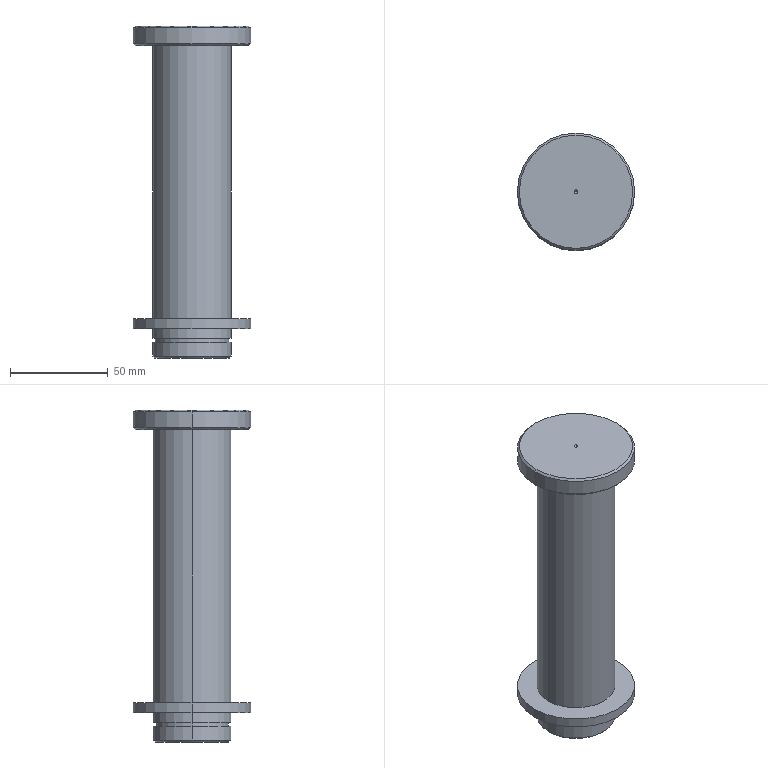Part | SolidWorks | features BaseBody 2 | 2 solids | 29 faces | box 60 x 60 x 170 mm | volume 236636 mm3 | cylinder 12 | cone 10 | plane 7 | commonest cylinder face diameters 40 x6 60 x4 37.5 x2
STEP:
#1=CARTESIAN_POINT('',(20.,0.,-89.));
#2=VERTEX_POINT('',#1);
#3=CARTESIAN_POINT('',(-20.,0.,-89.));
#4=VERTEX_POINT('',#3);
#5=CARTESIAN_POINT('',(0.,0.,-89.));
#6=DIRECTION('',(0.,0.,1.));
#7=DIRECTION('',(1.,0.,0.));
#8=AXIS2_PLACEMENT_3D('',#5,#6,#7);
#9=CIRCLE('',#8,20.);
#10=EDGE_CURVE('',#2,#4,#9,.T.);
#11=ORIENTED_EDGE('',*,*,#10,.T.);
#12=CARTESIAN_POINT('',(-20.,0.,-82.));
#13=VERTEX_POINT('',#12);
#14=CARTESIAN_POINT('',(-20.,0.,79.));
#15=DIRECTION('',(0.,0.,1.));
#16=VECTOR('',#15,1000.);
#17=LINE('',#14,#16);
#18=EDGE_CURVE('',#4,#13,#17,.T.);
#19=ORIENTED_EDGE('',*,*,#18,.T.);
#20=CARTESIAN_POINT('',(20.,0.,-82.));
#21=VERTEX_POINT('',#20);
#22=CARTESIAN_POINT('',(0.,0.,-82.));
#23=DIRECTION('',(0.,0.,1.));
#24=DIRECTION('',(1.,0.,0.));
#25=AXIS2_PLACEMENT_3D('',#22,#23,#24);
#26=CIRCLE('',#25,20.);
#27=EDGE_CURVE('',#21,#13,#26,.T.);
#28=ORIENTED_EDGE('',*,*,#27,.F.);
#29=CARTESIAN_POINT('',(20.,0.,79.));
#30=DIRECTION('',(0.,0.,1.));
#31=VECTOR('',#30,1000.);
#32=LINE('',#29,#31);
#33=EDGE_CURVE('',#2,#21,#32,.T.);
#34=ORIENTED_EDGE('',*,*,#33,.F.);
#35=EDGE_LOOP('',(#11,#19,#28,#34));
#36=FACE_OUTER_BOUND('',#35,.T.);
#37=CARTESIAN_POINT('',(0.,0.,79.));
#38=DIRECTION('',(0.,0.,1.));
#39=DIRECTION('',(1.,0.,0.));
#40=AXIS2_PLACEMENT_3D('',#37,#38,#39);
#41=CYLINDRICAL_SURFACE('',#40,20.);
#42=ADVANCED_FACE('',(#36),#41,.T.);
#43=CARTESIAN_POINT('',(19.,0.,-90.));
#44=VERTEX_POINT('',#43);
#45=CARTESIAN_POINT('',(-19.,0.,-90.));
#46=VERTEX_POINT('',#45);
#47=CARTESIAN_POINT('',(0.,0.,-90.));
#48=DIRECTION('',(0.,0.,1.));
#49=DIRECTION('',(1.,0.,0.));
#50=AXIS2_PLACEMENT_3D('',#47,#48,#49);
#51=CIRCLE('',#50,19.);
#52=EDGE_CURVE('',#44,#46,#51,.T.);
#53=ORIENTED_EDGE('',*,*,#52,.T.);
#54=CARTESIAN_POINT('',(-19.,0.,-90.));
#55=DIRECTION('',(-0.7071,0.,0.7071));
#56=VECTOR('',#55,1000.);
#57=LINE('',#54,#56);
#58=EDGE_CURVE('',#46,#4,#57,.T.);
#59=ORIENTED_EDGE('',*,*,#58,.T.);
#60=ORIENTED_EDGE('',*,*,#10,.F.);
#61=CARTESIAN_POINT('',(19.,0.,-90.));
#62=DIRECTION('',(0.7071,0.,0.7071));
#63=VECTOR('',#62,1000.);
#64=LINE('',#61,#63);
#65=EDGE_CURVE('',#44,#2,#64,.T.);
#66=ORIENTED_EDGE('',*,*,#65,.F.);
#67=EDGE_LOOP('',(#53,#59,#60,#66));
#68=FACE_OUTER_BOUND('',#67,.T.);
#69=CARTESIAN_POINT('',(0.,0.,-90.));
#70=DIRECTION('',(0.,0.,1.));
#71=DIRECTION('',(1.,0.,0.));
#72=AXIS2_PLACEMENT_3D('',#69,#70,#71);
#73=CONICAL_SURFACE('',#72,19.,0.7854);
#74=ADVANCED_FACE('',(#68),#73,.T.);
#75=CARTESIAN_POINT('',(0.,0.,-89.));
#76=VERTEX_POINT('',#75);
#77=CARTESIAN_POINT('',(-1.,0.,-90.));
#78=VERTEX_POINT('',#77);
#79=CARTESIAN_POINT('',(0.,0.,-89.));
#80=DIRECTION('',(-0.7071,0.,-0.7071));
#81=VECTOR('',#80,1000.);
#82=LINE('',#79,#81);
#83=EDGE_CURVE('',#76,#78,#82,.T.);
#84=ORIENTED_EDGE('',*,*,#83,.F.);
#85=CARTESIAN_POINT('',(1.,0.,-90.));
#86=VERTEX_POINT('',#85);
#87=CARTESIAN_POINT('',(0.,0.,-89.));
#88=DIRECTION('',(0.7071,0.,-0.7071));
#89=VECTOR('',#88,1000.);
#90=LINE('',#87,#89);
#91=EDGE_CURVE('',#76,#86,#90,.T.);
#92=ORIENTED_EDGE('',*,*,#91,.T.);
#93=CARTESIAN_POINT('',(0.,0.,-90.));
#94=DIRECTION('',(0.,0.,1.));
#95=DIRECTION('',(1.,0.,0.));
#96=AXIS2_PLACEMENT_3D('',#93,#94,#95);
#97=CIRCLE('',#96,1.);
#98=EDGE_CURVE('',#78,#86,#97,.T.);
#99=ORIENTED_EDGE('',*,*,#98,.F.);
#100=EDGE_LOOP('',(#84,#92,#99));
#101=FACE_OUTER_BOUND('',#100,.T.);
#102=CARTESIAN_POINT('',(0.,0.,-1089.));
#103=DIRECTION('',(0.,0.,-1.));
#104=DIRECTION('',(-1.,0.,0.));
#105=AXIS2_PLACEMENT_3D('',#102,#103,#104);
#106=CONICAL_SURFACE('',#105,1000.,0.7854);
#107=ADVANCED_FACE('',(#101),#106,.F.);
#108=CARTESIAN_POINT('',(0.,0.,79.));
#109=VERTEX_POINT('',#108);
#110=CARTESIAN_POINT('',(1.,0.,80.));
#111=VERTEX_POINT('',#110);
#112=CARTESIAN_POINT('',(1.,0.,80.));
#113=DIRECTION('',(0.7071,0.,0.7071));
#114=VECTOR('',#113,1000.);
#115=LINE('',#112,#114);
#116=EDGE_CURVE('',#109,#111,#115,.T.);
#117=ORIENTED_EDGE('',*,*,#116,.F.);
#118=CARTESIAN_POINT('',(-1.,0.,80.));
#119=VERTEX_POINT('',#118);
#120=CARTESIAN_POINT('',(-1.,0.,80.));
#121=DIRECTION('',(-0.7071,0.,0.7071));
#122=VECTOR('',#121,1000.);
#123=LINE('',#120,#122);
#124=EDGE_CURVE('',#109,#119,#123,.T.);
#125=ORIENTED_EDGE('',*,*,#124,.T.);
#126=CARTESIAN_POINT('',(0.,0.,80.));
#127=DIRECTION('',(0.,0.,1.));
#128=DIRECTION('',(1.,0.,0.));
#129=AXIS2_PLACEMENT_3D('',#126,#127,#128);
#130=CIRCLE('',#129,1.);
#131=EDGE_CURVE('',#119,#111,#130,.T.);
#132=ORIENTED_EDGE('',*,*,#131,.T.);
#133=EDGE_LOOP('',(#117,#125,#132));
#134=FACE_OUTER_BOUND('',#133,.T.);
#135=CARTESIAN_POINT('',(0.,0.,80.));
#136=DIRECTION('',(0.,0.,1.));
#137=DIRECTION('',(1.,0.,0.));
#138=AXIS2_PLACEMENT_3D('',#135,#136,#137);
#139=CONICAL_SURFACE('',#138,1.,0.7854);
#140=ADVANCED_FACE('',(#134),#139,.F.);
#141=CARTESIAN_POINT('',(29.,0.,80.));
#142=VERTEX_POINT('',#141);
#143=CARTESIAN_POINT('',(-29.,0.,80.));
#144=VERTEX_POINT('',#143);
#145=CARTESIAN_POINT('',(0.,0.,80.));
#146=DIRECTION('',(0.,0.,1.));
#147=DIRECTION('',(1.,0.,0.));
#148=AXIS2_PLACEMENT_3D('',#145,#146,#147);
#149=CIRCLE('',#148,29.);
#150=EDGE_CURVE('',#142,#144,#149,.T.);
#151=ORIENTED_EDGE('',*,*,#150,.F.);
#152=CARTESIAN_POINT('',(30.,0.,79.));
#153=VERTEX_POINT('',#152);
#154=CARTESIAN_POINT('',(30.,0.,79.));
#155=DIRECTION('',(0.7071,0.,-0.7071));
#156=VECTOR('',#155,1000.);
#157=LINE('',#154,#156);
#158=EDGE_CURVE('',#142,#153,#157,.T.);
#159=ORIENTED_EDGE('',*,*,#158,.T.);
#160=CARTESIAN_POINT('',(-30.,0.,79.));
#161=VERTEX_POINT('',#160);
#162=CARTESIAN_POINT('',(0.,0.,79.));
#163=DIRECTION('',(0.,0.,1.));
#164=DIRECTION('',(1.,0.,0.));
#165=AXIS2_PLACEMENT_3D('',#162,#163,#164);
#166=CIRCLE('',#165,30.);
#167=EDGE_CURVE('',#153,#161,#166,.T.);
#168=ORIENTED_EDGE('',*,*,#167,.T.);
#169=CARTESIAN_POINT('',(-30.,0.,79.));
#170=DIRECTION('',(-0.7071,0.,-0.7071));
#171=VECTOR('',#170,1000.);
#172=LINE('',#169,#171);
#173=EDGE_CURVE('',#144,#161,#172,.T.);
#174=ORIENTED_EDGE('',*,*,#173,.F.);
#175=EDGE_LOOP('',(#151,#159,#168,#174));
#176=FACE_OUTER_BOUND('',#175,.T.);
#177=CARTESIAN_POINT('',(0.,0.,79.));
#178=DIRECTION('',(0.,0.,-1.));
#179=DIRECTION('',(-1.,0.,0.));
#180=AXIS2_PLACEMENT_3D('',#177,#178,#179);
#181=CONICAL_SURFACE('',#180,30.,0.7854);
#182=ADVANCED_FACE('',(#176),#181,.T.);
#183=CARTESIAN_POINT('',(30.,0.,71.));
#184=VERTEX_POINT('',#183);
#185=CARTESIAN_POINT('',(-30.,0.,71.));
#186=VERTEX_POINT('',#185);
#187=CARTESIAN_POINT('',(0.,0.,71.));
#188=DIRECTION('',(0.,0.,1.));
#189=DIRECTION('',(1.,0.,0.));
#190=AXIS2_PLACEMENT_3D('',#187,#188,#189);
#191=CIRCLE('',#190,30.);
#192=EDGE_CURVE('',#184,#186,#191,.T.);
#193=ORIENTED_EDGE('',*,*,#192,.T.);
#194=CARTESIAN_POINT('',(-30.,0.,79.));
#195=DIRECTION('',(0.,0.,1.));
#196=VECTOR('',#195,1000.);
#197=LINE('',#194,#196);
#198=EDGE_CURVE('',#186,#161,#197,.T.);
#199=ORIENTED_EDGE('',*,*,#198,.T.);
#200=ORIENTED_EDGE('',*,*,#167,.F.);
#201=CARTESIAN_POINT('',(30.,0.,79.));
#202=DIRECTION('',(0.,0.,1.));
#203=VECTOR('',#202,1000.);
#204=LINE('',#201,#203);
#205=EDGE_CURVE('',#184,#153,#204,.T.);
#206=ORIENTED_EDGE('',*,*,#205,.F.);
#207=EDGE_LOOP('',(#193,#199,#200,#206));
#208=FACE_OUTER_BOUND('',#207,.T.);
#209=CARTESIAN_POINT('',(0.,0.,79.));
#210=DIRECTION('',(0.,0.,1.));
#211=DIRECTION('',(1.,0.,0.));
#212=AXIS2_PLACEMENT_3D('',#209,#210,#211);
#213=CYLINDRICAL_SURFACE('',#212,30.);
#214=ADVANCED_FACE('',(#208),#213,.T.);
#215=CARTESIAN_POINT('',(29.,0.,70.));
#216=VERTEX_POINT('',#215);
#217=CARTESIAN_POINT('',(-29.,0.,70.));
#218=VERTEX_POINT('',#217);
#219=CARTESIAN_POINT('',(0.,0.,70.));
#220=DIRECTION('',(0.,0.,1.));
#221=DIRECTION('',(1.,0.,0.));
#222=AXIS2_PLACEMENT_3D('',#219,#220,#221);
#223=CIRCLE('',#222,29.);
#224=EDGE_CURVE('',#216,#218,#223,.T.);
#225=ORIENTED_EDGE('',*,*,#224,.T.);
#226=CARTESIAN_POINT('',(-29.,0.,70.));
#227=DIRECTION('',(-0.7071,0.,0.7071));
#228=VECTOR('',#227,1000.);
#229=LINE('',#226,#228);
#230=EDGE_CURVE('',#218,#186,#229,.T.);
#231=ORIENTED_EDGE('',*,*,#230,.T.);
#232=ORIENTED_EDGE('',*,*,#192,.F.);
#233=CARTESIAN_POINT('',(29.,0.,70.));
#234=DIRECTION('',(0.7071,0.,0.7071));
#235=VECTOR('',#234,1000.);
#236=LINE('',#233,#235);
#237=EDGE_CURVE('',#216,#184,#236,.T.);
#238=ORIENTED_EDGE('',*,*,#237,.F.);
#239=EDGE_LOOP('',(#225,#231,#232,#238));
#240=FACE_OUTER_BOUND('',#239,.T.);
#241=CARTESIAN_POINT('',(0.,0.,70.));
#242=DIRECTION('',(0.,0.,1.));
#243=DIRECTION('',(1.,0.,0.));
#244=AXIS2_PLACEMENT_3D('',#241,#242,#243);
#245=CONICAL_SURFACE('',#244,29.,0.7854);
#246=ADVANCED_FACE('',(#240),#245,.T.);
#247=CARTESIAN_POINT('',(20.,0.,-80.));
#248=VERTEX_POINT('',#247);
#249=CARTESIAN_POINT('',(-20.,0.,-80.));
#250=VERTEX_POINT('',#249);
#251=CARTESIAN_POINT('',(0.,0.,-80.));
#252=DIRECTION('',(0.,0.,1.));
#253=DIRECTION('',(1.,0.,0.));
#254=AXIS2_PLACEMENT_3D('',#251,#252,#253);
#255=CIRCLE('',#254,20.);
#256=EDGE_CURVE('',#248,#250,#255,.T.);
#257=ORIENTED_EDGE('',*,*,#256,.T.);
#258=CARTESIAN_POINT('',(-20.,0.,70.));
#259=VERTEX_POINT('',#258);
#260=CARTESIAN_POINT('',(-20.,0.,79.));
#261=DIRECTION('',(0.,0.,1.));
#262=VECTOR('',#261,1000.);
#263=LINE('',#260,#262);
#264=EDGE_CURVE('',#250,#259,#263,.T.);
#265=ORIENTED_EDGE('',*,*,#264,.T.);
#266=CARTESIAN_POINT('',(20.,0.,70.));
#267=VERTEX_POINT('',#266);
#268=CARTESIAN_POINT('',(0.,0.,70.));
#269=DIRECTION('',(0.,0.,1.));
#270=DIRECTION('',(1.,0.,0.));
#271=AXIS2_PLACEMENT_3D('',#268,#269,#270);
#272=CIRCLE('',#271,20.);
#273=EDGE_CURVE('',#267,#259,#272,.T.);
#274=ORIENTED_EDGE('',*,*,#273,.F.);
#275=CARTESIAN_POINT('',(20.,0.,79.));
#276=DIRECTION('',(0.,0.,1.));
#277=VECTOR('',#276,1000.);
#278=LINE('',#275,#277);
#279=EDGE_CURVE('',#248,#267,#278,.T.);
#280=ORIENTED_EDGE('',*,*,#279,.F.);
#281=EDGE_LOOP('',(#257,#265,#274,#280));
#282=FACE_OUTER_BOUND('',#281,.T.);
#283=CARTESIAN_POINT('',(0.,0.,79.));
#284=DIRECTION('',(0.,0.,1.));
#285=DIRECTION('',(1.,0.,0.));
#286=AXIS2_PLACEMENT_3D('',#283,#284,#285);
#287=CYLINDRICAL_SURFACE('',#286,20.);
#288=ADVANCED_FACE('',(#282),#287,.T.);
#289=CARTESIAN_POINT('',(18.75,0.,-82.));
#290=VERTEX_POINT('',#289);
#291=CARTESIAN_POINT('',(-18.75,0.,-82.));
#292=VERTEX_POINT('',#291);
#293=CARTESIAN_POINT('',(0.,0.,-82.));
#294=DIRECTION('',(0.,0.,1.));
#295=DIRECTION('',(1.,0.,0.));
#296=AXIS2_PLACEMENT_3D('',#293,#294,#295);
#297=CIRCLE('',#296,18.75);
#298=EDGE_CURVE('',#290,#292,#297,.T.);
#299=ORIENTED_EDGE('',*,*,#298,.T.);
#300=CARTESIAN_POINT('',(-18.75,0.,-80.));
#301=VERTEX_POINT('',#300);
#302=CARTESIAN_POINT('',(-18.75,0.,79.));
#303=DIRECTION('',(0.,0.,1.));
#304=VECTOR('',#303,1000.);
#305=LINE('',#302,#304);
#306=EDGE_CURVE('',#292,#301,#305,.T.);
#307=ORIENTED_EDGE('',*,*,#306,.T.);
#308=CARTESIAN_POINT('',(18.75,0.,-80.));
#309=VERTEX_POINT('',#308);
#310=CARTESIAN_POINT('',(0.,0.,-80.));
#311=DIRECTION('',(0.,0.,1.));
#312=DIRECTION('',(1.,0.,0.));
#313=AXIS2_PLACEMENT_3D('',#310,#311,#312);
#314=CIRCLE('',#313,18.75);
#315=EDGE_CURVE('',#309,#301,#314,.T.);
#316=ORIENTED_EDGE('',*,*,#315,.F.);
#317=CARTESIAN_POINT('',(18.75,0.,79.));
#318=DIRECTION('',(0.,0.,1.));
#319=VECTOR('',#318,1000.);
#320=LINE('',#317,#319);
#321=EDGE_CURVE('',#290,#309,#320,.T.);
#322=ORIENTED_EDGE('',*,*,#321,.F.);
#323=EDGE_LOOP('',(#299,#307,#316,#322));
#324=FACE_OUTER_BOUND('',#323,.T.);
#325=CARTESIAN_POINT('',(0.,0.,79.));
#326=DIRECTION('',(0.,0.,1.));
#327=DIRECTION('',(1.,0.,0.));
#328=AXIS2_PLACEMENT_3D('',#325,#326,#327);
#329=CYLINDRICAL_SURFACE('',#328,18.75);
#330=ADVANCED_FACE('',(#324),#329,.T.);
#331=ORIENTED_EDGE('',*,*,#306,.F.);
#332=CARTESIAN_POINT('',(0.,0.,-82.));
#333=DIRECTION('',(0.,0.,1.));
#334=DIRECTION('',(1.,0.,0.));
#335=AXIS2_PLACEMENT_3D('',#332,#333,#334);
#336=CIRCLE('',#335,18.75);
#337=EDGE_CURVE('',#292,#290,#336,.T.);
#338=ORIENTED_EDGE('',*,*,#337,.T.);
#339=ORIENTED_EDGE('',*,*,#321,.T.);
#340=CARTESIAN_POINT('',(0.,0.,-80.));
#341=DIRECTION('',(0.,0.,1.));
#342=DIRECTION('',(1.,0.,0.));
#343=AXIS2_PLACEMENT_3D('',#340,#341,#342);
#344=CIRCLE('',#343,18.75);
#345=EDGE_CURVE('',#301,#309,#344,.T.);
#346=ORIENTED_EDGE('',*,*,#345,.F.);
#347=EDGE_LOOP('',(#331,#338,#339,#346));
#348=FACE_OUTER_BOUND('',#347,.T.);
#349=CARTESIAN_POINT('',(0.,0.,79.));
#350=DIRECTION('',(0.,0.,1.));
#351=DIRECTION('',(1.,0.,0.));
#352=AXIS2_PLACEMENT_3D('',#349,#350,#351);
#353=CYLINDRICAL_SURFACE('',#352,18.75);
#354=ADVANCED_FACE('',(#348),#353,.T.);
#355=ORIENTED_EDGE('',*,*,#256,.F.);
#356=CARTESIAN_POINT('',(0.,0.,-80.));
#357=DIRECTION('',(0.,0.,1.));
#358=DIRECTION('',(1.,0.,0.));
#359=AXIS2_PLACEMENT_3D('',#356,#357,#358);
#360=CIRCLE('',#359,20.);
#361=EDGE_CURVE('',#250,#248,#360,.T.);
#362=ORIENTED_EDGE('',*,*,#361,.F.);
#363=EDGE_LOOP('',(#355,#362));
#364=FACE_OUTER_BOUND('',#363,.T.);
#365=ORIENTED_EDGE('',*,*,#315,.T.);
#366=ORIENTED_EDGE('',*,*,#345,.T.);
#367=EDGE_LOOP('',(#365,#366));
#368=FACE_BOUND('',#367,.T.);
#369=CARTESIAN_POINT('',(0.,20.,-80.));
#370=DIRECTION('',(0.,0.,1.));
#371=DIRECTION('',(1.,0.,0.));
#372=AXIS2_PLACEMENT_3D('',#369,#370,#371);
#373=PLANE('',#372);
#374=ADVANCED_FACE('',(#364,#368),#373,.F.);
#375=ORIENTED_EDGE('',*,*,#264,.F.);
#376=ORIENTED_EDGE('',*,*,#361,.T.);
#377=ORIENTED_EDGE('',*,*,#279,.T.);
#378=CARTESIAN_POINT('',(0.,0.,70.));
#379=DIRECTION('',(0.,0.,1.));
#380=DIRECTION('',(1.,0.,0.));
#381=AXIS2_PLACEMENT_3D('',#378,#379,#380);
#382=CIRCLE('',#381,20.);
#383=EDGE_CURVE('',#259,#267,#382,.T.);
#384=ORIENTED_EDGE('',*,*,#383,.F.);
#385=EDGE_LOOP('',(#375,#376,#377,#384));
#386=FACE_OUTER_BOUND('',#385,.T.);
#387=CARTESIAN_POINT('',(0.,0.,79.));
#388=DIRECTION('',(0.,0.,1.));
#389=DIRECTION('',(1.,0.,0.));
#390=AXIS2_PLACEMENT_3D('',#387,#388,#389);
#391=CYLINDRICAL_SURFACE('',#390,20.);
#392=ADVANCED_FACE('',(#386),#391,.T.);
#393=ORIENTED_EDGE('',*,*,#224,.F.);
#394=CARTESIAN_POINT('',(0.,0.,70.));
#395=DIRECTION('',(0.,0.,1.));
#396=DIRECTION('',(1.,0.,0.));
#397=AXIS2_PLACEMENT_3D('',#394,#395,#396);
#398=CIRCLE('',#397,29.);
#399=EDGE_CURVE('',#218,#216,#398,.T.);
#400=ORIENTED_EDGE('',*,*,#399,.F.);
#401=EDGE_LOOP('',(#393,#400));
#402=FACE_OUTER_BOUND('',#401,.T.);
#403=ORIENTED_EDGE('',*,*,#273,.T.);
#404=ORIENTED_EDGE('',*,*,#383,.T.);
#405=EDGE_LOOP('',(#403,#404));
#406=FACE_BOUND('',#405,.T.);
#407=CARTESIAN_POINT('',(0.,29.,70.));
#408=DIRECTION('',(0.,0.,1.));
#409=DIRECTION('',(1.,0.,0.));
#410=AXIS2_PLACEMENT_3D('',#407,#408,#409);
#411=PLANE('',#410);
#412=ADVANCED_FACE('',(#402,#406),#411,.F.);
#413=ORIENTED_EDGE('',*,*,#230,.F.);
#414=ORIENTED_EDGE('',*,*,#399,.T.);
#415=ORIENTED_EDGE('',*,*,#237,.T.);
#416=CARTESIAN_POINT('',(0.,0.,71.));
#417=DIRECTION('',(0.,0.,1.));
#418=DIRECTION('',(1.,0.,0.));
#419=AXIS2_PLACEMENT_3D('',#416,#417,#418);
#420=CIRCLE('',#419,30.);
#421=EDGE_CURVE('',#186,#184,#420,.T.);
#422=ORIENTED_EDGE('',*,*,#421,.F.);
#423=EDGE_LOOP('',(#413,#414,#415,#422));
#424=FACE_OUTER_BOUND('',#423,.T.);
#425=CARTESIAN_POINT('',(0.,0.,70.));
#426=DIRECTION('',(0.,0.,1.));
#427=DIRECTION('',(1.,0.,0.));
#428=AXIS2_PLACEMENT_3D('',#425,#426,#427);
#429=CONICAL_SURFACE('',#428,29.,0.7854);
#430=ADVANCED_FACE('',(#424),#429,.T.);
#431=ORIENTED_EDGE('',*,*,#198,.F.);
#432=ORIENTED_EDGE('',*,*,#421,.T.);
#433=ORIENTED_EDGE('',*,*,#205,.T.);
#434=CARTESIAN_POINT('',(0.,0.,79.));
#435=DIRECTION('',(0.,0.,1.));
#436=DIRECTION('',(1.,0.,0.));
#437=AXIS2_PLACEMENT_3D('',#434,#435,#436);
#438=CIRCLE('',#437,30.);
#439=EDGE_CURVE('',#161,#153,#438,.T.);
#440=ORIENTED_EDGE('',*,*,#439,.F.);
#441=EDGE_LOOP('',(#431,#432,#433,#440));
#442=FACE_OUTER_BOUND('',#441,.T.);
#443=CARTESIAN_POINT('',(0.,0.,79.));
#444=DIRECTION('',(0.,0.,1.));
#445=DIRECTION('',(1.,0.,0.));
#446=AXIS2_PLACEMENT_3D('',#443,#444,#445);
#447=CYLINDRICAL_SURFACE('',#446,30.);
#448=ADVANCED_FACE('',(#442),#447,.T.);
#449=ORIENTED_EDGE('',*,*,#158,.F.);
#450=CARTESIAN_POINT('',(0.,0.,80.));
#451=DIRECTION('',(0.,0.,1.));
#452=DIRECTION('',(1.,0.,0.));
#453=AXIS2_PLACEMENT_3D('',#450,#451,#452);
#454=CIRCLE('',#453,29.);
#455=EDGE_CURVE('',#144,#142,#454,.T.);
#456=ORIENTED_EDGE('',*,*,#455,.F.);
#457=ORIENTED_EDGE('',*,*,#173,.T.);
#458=ORIENTED_EDGE('',*,*,#439,.T.);
#459=EDGE_LOOP('',(#449,#456,#457,#458));
#460=FACE_OUTER_BOUND('',#459,.T.);
#461=CARTESIAN_POINT('',(0.,0.,79.));
#462=DIRECTION('',(0.,0.,-1.));
#463=DIRECTION('',(-1.,0.,0.));
#464=AXIS2_PLACEMENT_3D('',#461,#462,#463);
#465=CONICAL_SURFACE('',#464,30.,0.7854);
#466=ADVANCED_FACE('',(#460),#465,.T.);
#467=CARTESIAN_POINT('',(0.,0.,80.));
#468=DIRECTION('',(0.,0.,1.));
#469=DIRECTION('',(1.,0.,0.));
#470=AXIS2_PLACEMENT_3D('',#467,#468,#469);
#471=CIRCLE('',#470,1.);
#472=EDGE_CURVE('',#111,#119,#471,.T.);
#473=ORIENTED_EDGE('',*,*,#472,.F.);
#474=ORIENTED_EDGE('',*,*,#131,.F.);
#475=EDGE_LOOP('',(#473,#474));
#476=FACE_BOUND('',#475,.T.);
#477=ORIENTED_EDGE('',*,*,#455,.T.);
#478=ORIENTED_EDGE('',*,*,#150,.T.);
#479=EDGE_LOOP('',(#477,#478));
#480=FACE_OUTER_BOUND('',#479,.T.);
#481=CARTESIAN_POINT('',(0.,1.,80.));
#482=DIRECTION('',(0.,0.,-1.));
#483=DIRECTION('',(-1.,0.,0.));
#484=AXIS2_PLACEMENT_3D('',#481,#482,#483);
#485=PLANE('',#484);
#486=ADVANCED_FACE('',(#476,#480),#485,.F.);
#487=ORIENTED_EDGE('',*,*,#124,.F.);
#488=ORIENTED_EDGE('',*,*,#116,.T.);
#489=ORIENTED_EDGE('',*,*,#472,.T.);
#490=EDGE_LOOP('',(#487,#488,#489));
#491=FACE_OUTER_BOUND('',#490,.T.);
#492=CARTESIAN_POINT('',(0.,0.,80.));
#493=DIRECTION('',(0.,0.,1.));
#494=DIRECTION('',(1.,0.,0.));
#495=AXIS2_PLACEMENT_3D('',#492,#493,#494);
#496=CONICAL_SURFACE('',#495,1.,0.7854);
#497=ADVANCED_FACE('',(#491),#496,.F.);
#498=ORIENTED_EDGE('',*,*,#91,.F.);
#499=ORIENTED_EDGE('',*,*,#83,.T.);
#500=CARTESIAN_POINT('',(0.,0.,-90.));
#501=DIRECTION('',(0.,0.,1.));
#502=DIRECTION('',(1.,0.,0.));
#503=AXIS2_PLACEMENT_3D('',#500,#501,#502);
#504=CIRCLE('',#503,1.);
#505=EDGE_CURVE('',#86,#78,#504,.T.);
#506=ORIENTED_EDGE('',*,*,#505,.F.);
#507=EDGE_LOOP('',(#498,#499,#506));
#508=FACE_OUTER_BOUND('',#507,.T.);
#509=CARTESIAN_POINT('',(0.,0.,-1089.));
#510=DIRECTION('',(0.,0.,-1.));
#511=DIRECTION('',(-1.,0.,0.));
#512=AXIS2_PLACEMENT_3D('',#509,#510,#511);
#513=CONICAL_SURFACE('',#512,1000.,0.7854);
#514=ADVANCED_FACE('',(#508),#513,.F.);
#515=ORIENTED_EDGE('',*,*,#52,.F.);
#516=CARTESIAN_POINT('',(0.,0.,-90.));
#517=DIRECTION('',(0.,0.,1.));
#518=DIRECTION('',(1.,0.,0.));
#519=AXIS2_PLACEMENT_3D('',#516,#517,#518);
#520=CIRCLE('',#519,19.);
#521=EDGE_CURVE('',#46,#44,#520,.T.);
#522=ORIENTED_EDGE('',*,*,#521,.F.);
#523=EDGE_LOOP('',(#515,#522));
#524=FACE_OUTER_BOUND('',#523,.T.);
#525=ORIENTED_EDGE('',*,*,#98,.T.);
#526=ORIENTED_EDGE('',*,*,#505,.T.);
#527=EDGE_LOOP('',(#525,#526));
#528=FACE_BOUND('',#527,.T.);
#529=CARTESIAN_POINT('',(0.,19.,-90.));
#530=DIRECTION('',(0.,0.,1.));
#531=DIRECTION('',(1.,0.,0.));
#532=AXIS2_PLACEMENT_3D('',#529,#530,#531);
#533=PLANE('',#532);
#534=ADVANCED_FACE('',(#524,#528),#533,.F.);
#535=ORIENTED_EDGE('',*,*,#58,.F.);
#536=ORIENTED_EDGE('',*,*,#521,.T.);
#537=ORIENTED_EDGE('',*,*,#65,.T.);
#538=CARTESIAN_POINT('',(0.,0.,-89.));
#539=DIRECTION('',(0.,0.,1.));
#540=DIRECTION('',(1.,0.,0.));
#541=AXIS2_PLACEMENT_3D('',#538,#539,#540);
#542=CIRCLE('',#541,20.);
#543=EDGE_CURVE('',#4,#2,#542,.T.);
#544=ORIENTED_EDGE('',*,*,#543,.F.);
#545=EDGE_LOOP('',(#535,#536,#537,#544));
#546=FACE_OUTER_BOUND('',#545,.T.);
#547=CARTESIAN_POINT('',(0.,0.,-90.));
#548=DIRECTION('',(0.,0.,1.));
#549=DIRECTION('',(1.,0.,0.));
#550=AXIS2_PLACEMENT_3D('',#547,#548,#549);
#551=CONICAL_SURFACE('',#550,19.,0.7854);
#552=ADVANCED_FACE('',(#546),#551,.T.);
#553=ORIENTED_EDGE('',*,*,#18,.F.);
#554=ORIENTED_EDGE('',*,*,#543,.T.);
#555=ORIENTED_EDGE('',*,*,#33,.T.);
#556=CARTESIAN_POINT('',(0.,0.,-82.));
#557=DIRECTION('',(0.,0.,1.));
#558=DIRECTION('',(1.,0.,0.));
#559=AXIS2_PLACEMENT_3D('',#556,#557,#558);
#560=CIRCLE('',#559,20.);
#561=EDGE_CURVE('',#13,#21,#560,.T.);
#562=ORIENTED_EDGE('',*,*,#561,.F.);
#563=EDGE_LOOP('',(#553,#554,#555,#562));
#564=FACE_OUTER_BOUND('',#563,.T.);
#565=CARTESIAN_POINT('',(0.,0.,79.));
#566=DIRECTION('',(0.,0.,1.));
#567=DIRECTION('',(1.,0.,0.));
#568=AXIS2_PLACEMENT_3D('',#565,#566,#567);
#569=CYLINDRICAL_SURFACE('',#568,20.);
#570=ADVANCED_FACE('',(#564),#569,.T.);
#571=ORIENTED_EDGE('',*,*,#298,.F.);
#572=ORIENTED_EDGE('',*,*,#337,.F.);
#573=EDGE_LOOP('',(#571,#572));
#574=FACE_BOUND('',#573,.T.);
#575=ORIENTED_EDGE('',*,*,#27,.T.);
#576=ORIENTED_EDGE('',*,*,#561,.T.);
#577=EDGE_LOOP('',(#575,#576));
#578=FACE_OUTER_BOUND('',#577,.T.);
#579=CARTESIAN_POINT('',(0.,18.75,-82.));
#580=DIRECTION('',(0.,0.,-1.));
#581=DIRECTION('',(-1.,0.,0.));
#582=AXIS2_PLACEMENT_3D('',#579,#580,#581);
#583=PLANE('',#582);
#584=ADVANCED_FACE('',(#574,#578),#583,.F.);
#585=CLOSED_SHELL('',(#42,#74,#107,#140,#182,#214,#246,#288,#330,#354,#374,#392,#412,#430,#448,#466,#486,#497,#514,#534,#552,#570,#584));
#586=MANIFOLD_SOLID_BREP('',#585);
#587=CARTESIAN_POINT('',(20.,0.,-70.));
#588=VERTEX_POINT('',#587);
#589=CARTESIAN_POINT('',(-20.,0.,-70.));
#590=VERTEX_POINT('',#589);
#591=CARTESIAN_POINT('',(0.,0.,-70.));
#592=DIRECTION('',(0.,0.,-1.));
#593=DIRECTION('',(-1.,0.,0.));
#594=AXIS2_PLACEMENT_3D('',#591,#592,#593);
#595=CIRCLE('',#594,20.);
#596=EDGE_CURVE('',#588,#590,#595,.T.);
#597=ORIENTED_EDGE('',*,*,#596,.F.);
#598=CARTESIAN_POINT('',(20.,0.,-75.));
#599=VERTEX_POINT('',#598);
#600=CARTESIAN_POINT('',(20.,0.,-70.));
#601=DIRECTION('',(0.,0.,-1.));
#602=VECTOR('',#601,1000.);
#603=LINE('',#600,#602);
#604=EDGE_CURVE('',#588,#599,#603,.T.);
#605=ORIENTED_EDGE('',*,*,#604,.T.);
#606=CARTESIAN_POINT('',(-20.,0.,-75.));
#607=VERTEX_POINT('',#606);
#608=CARTESIAN_POINT('',(0.,0.,-75.));
#609=DIRECTION('',(0.,0.,-1.));
#610=DIRECTION('',(-1.,0.,0.));
#611=AXIS2_PLACEMENT_3D('',#608,#609,#610);
#612=CIRCLE('',#611,20.);
#613=EDGE_CURVE('',#599,#607,#612,.T.);
#614=ORIENTED_EDGE('',*,*,#613,.T.);
#615=CARTESIAN_POINT('',(-20.,0.,-70.));
#616=DIRECTION('',(0.,0.,-1.));
#617=VECTOR('',#616,1000.);
#618=LINE('',#615,#617);
#619=EDGE_CURVE('',#590,#607,#618,.T.);
#620=ORIENTED_EDGE('',*,*,#619,.F.);
#621=EDGE_LOOP('',(#597,#605,#614,#620));
#622=FACE_OUTER_BOUND('',#621,.T.);
#623=CARTESIAN_POINT('',(0.,0.,-70.));
#624=DIRECTION('',(0.,0.,-1.));
#625=DIRECTION('',(-1.,0.,0.));
#626=AXIS2_PLACEMENT_3D('',#623,#624,#625);
#627=CYLINDRICAL_SURFACE('',#626,20.);
#628=ADVANCED_FACE('',(#622),#627,.F.);
#629=CARTESIAN_POINT('',(-30.,0.,-70.));
#630=VERTEX_POINT('',#629);
#631=CARTESIAN_POINT('',(30.,0.,-70.));
#632=VERTEX_POINT('',#631);
#633=CARTESIAN_POINT('',(0.,0.,-70.));
#634=DIRECTION('',(0.,0.,-1.));
#635=DIRECTION('',(-1.,0.,0.));
#636=AXIS2_PLACEMENT_3D('',#633,#634,#635);
#637=CIRCLE('',#636,30.);
#638=EDGE_CURVE('',#630,#632,#637,.T.);
#639=ORIENTED_EDGE('',*,*,#638,.T.);
#640=CARTESIAN_POINT('',(30.,0.,-75.));
#641=VERTEX_POINT('',#640);
#642=CARTESIAN_POINT('',(30.,0.,-70.));
#643=DIRECTION('',(0.,0.,-1.));
#644=VECTOR('',#643,1000.);
#645=LINE('',#642,#644);
#646=EDGE_CURVE('',#632,#641,#645,.T.);
#647=ORIENTED_EDGE('',*,*,#646,.T.);
#648=CARTESIAN_POINT('',(-30.,0.,-75.));
#649=VERTEX_POINT('',#648);
#650=CARTESIAN_POINT('',(0.,0.,-75.));
#651=DIRECTION('',(0.,0.,-1.));
#652=DIRECTION('',(-1.,0.,0.));
#653=AXIS2_PLACEMENT_3D('',#650,#651,#652);
#654=CIRCLE('',#653,30.);
#655=EDGE_CURVE('',#649,#641,#654,.T.);
#656=ORIENTED_EDGE('',*,*,#655,.F.);
#657=CARTESIAN_POINT('',(-30.,0.,-70.));
#658=DIRECTION('',(0.,0.,-1.));
#659=VECTOR('',#658,1000.);
#660=LINE('',#657,#659);
#661=EDGE_CURVE('',#630,#649,#660,.T.);
#662=ORIENTED_EDGE('',*,*,#661,.F.);
#663=EDGE_LOOP('',(#639,#647,#656,#662));
#664=FACE_OUTER_BOUND('',#663,.T.);
#665=CARTESIAN_POINT('',(0.,0.,-70.));
#666=DIRECTION('',(0.,0.,-1.));
#667=DIRECTION('',(-1.,0.,0.));
#668=AXIS2_PLACEMENT_3D('',#665,#666,#667);
#669=CYLINDRICAL_SURFACE('',#668,30.);
#670=ADVANCED_FACE('',(#664),#669,.T.);
#671=ORIENTED_EDGE('',*,*,#646,.F.);
#672=CARTESIAN_POINT('',(0.,0.,-70.));
#673=DIRECTION('',(0.,0.,-1.));
#674=DIRECTION('',(-1.,0.,0.));
#675=AXIS2_PLACEMENT_3D('',#672,#673,#674);
#676=CIRCLE('',#675,30.);
#677=EDGE_CURVE('',#632,#630,#676,.T.);
#678=ORIENTED_EDGE('',*,*,#677,.T.);
#679=ORIENTED_EDGE('',*,*,#661,.T.);
#680=CARTESIAN_POINT('',(0.,0.,-75.));
#681=DIRECTION('',(0.,0.,-1.));
#682=DIRECTION('',(-1.,0.,0.));
#683=AXIS2_PLACEMENT_3D('',#680,#681,#682);
#684=CIRCLE('',#683,30.);
#685=EDGE_CURVE('',#641,#649,#684,.T.);
#686=ORIENTED_EDGE('',*,*,#685,.F.);
#687=EDGE_LOOP('',(#671,#678,#679,#686));
#688=FACE_OUTER_BOUND('',#687,.T.);
#689=CARTESIAN_POINT('',(0.,0.,-70.));
#690=DIRECTION('',(0.,0.,-1.));
#691=DIRECTION('',(-1.,0.,0.));
#692=AXIS2_PLACEMENT_3D('',#689,#690,#691);
#693=CYLINDRICAL_SURFACE('',#692,30.);
#694=ADVANCED_FACE('',(#688),#693,.T.);
#695=CARTESIAN_POINT('',(0.,0.,-70.));
#696=DIRECTION('',(0.,0.,-1.));
#697=DIRECTION('',(-1.,0.,0.));
#698=AXIS2_PLACEMENT_3D('',#695,#696,#697);
#699=CIRCLE('',#698,20.);
#700=EDGE_CURVE('',#590,#588,#699,.T.);
#701=ORIENTED_EDGE('',*,*,#700,.T.);
#702=ORIENTED_EDGE('',*,*,#596,.T.);
#703=EDGE_LOOP('',(#701,#702));
#704=FACE_BOUND('',#703,.T.);
#705=ORIENTED_EDGE('',*,*,#638,.F.);
#706=ORIENTED_EDGE('',*,*,#677,.F.);
#707=EDGE_LOOP('',(#705,#706));
#708=FACE_OUTER_BOUND('',#707,.T.);
#709=CARTESIAN_POINT('',(0.,0.,-70.));
#710=DIRECTION('',(0.,0.,-1.));
#711=DIRECTION('',(-1.,0.,0.));
#712=AXIS2_PLACEMENT_3D('',#709,#710,#711);
#713=PLANE('',#712);
#714=ADVANCED_FACE('',(#704,#708),#713,.F.);
#715=CARTESIAN_POINT('',(0.,0.,-75.));
#716=DIRECTION('',(0.,0.,-1.));
#717=DIRECTION('',(-1.,0.,0.));
#718=AXIS2_PLACEMENT_3D('',#715,#716,#717);
#719=CIRCLE('',#718,20.);
#720=EDGE_CURVE('',#607,#599,#719,.T.);
#721=ORIENTED_EDGE('',*,*,#720,.F.);
#722=ORIENTED_EDGE('',*,*,#613,.F.);
#723=EDGE_LOOP('',(#721,#722));
#724=FACE_BOUND('',#723,.T.);
#725=ORIENTED_EDGE('',*,*,#655,.T.);
#726=ORIENTED_EDGE('',*,*,#685,.T.);
#727=EDGE_LOOP('',(#725,#726));
#728=FACE_OUTER_BOUND('',#727,.T.);
#729=CARTESIAN_POINT('',(0.,0.,-75.));
#730=DIRECTION('',(0.,0.,-1.));
#731=DIRECTION('',(-1.,0.,0.));
#732=AXIS2_PLACEMENT_3D('',#729,#730,#731);
#733=PLANE('',#732);
#734=ADVANCED_FACE('',(#724,#728),#733,.T.);
#735=ORIENTED_EDGE('',*,*,#604,.F.);
#736=ORIENTED_EDGE('',*,*,#700,.F.);
#737=ORIENTED_EDGE('',*,*,#619,.T.);
#738=ORIENTED_EDGE('',*,*,#720,.T.);
#739=EDGE_LOOP('',(#735,#736,#737,#738));
#740=FACE_OUTER_BOUND('',#739,.T.);
#741=CARTESIAN_POINT('',(0.,0.,-70.));
#742=DIRECTION('',(0.,0.,-1.));
#743=DIRECTION('',(-1.,0.,0.));
#744=AXIS2_PLACEMENT_3D('',#741,#742,#743);
#745=CYLINDRICAL_SURFACE('',#744,20.);
#746=ADVANCED_FACE('',(#740),#745,.F.);
#747=CLOSED_SHELL('',(#628,#670,#694,#714,#734,#746));
#748=MANIFOLD_SOLID_BREP('',#747);
#749=CARTESIAN_POINT('',(0.,0.,0.));
#750=DIRECTION('',(0.,0.,1.));
#751=DIRECTION('',(1.,0.,0.));
#752=AXIS2_PLACEMENT_3D('',#749,#750,#751);
#753=(LENGTH_UNIT()NAMED_UNIT(*)SI_UNIT(.MILLI.,.METRE.));
#754=UNCERTAINTY_MEASURE_WITH_UNIT(LENGTH_MEASURE(0.00001),#753,'','');
#755=(NAMED_UNIT(*)PLANE_ANGLE_UNIT()SI_UNIT($,.RADIAN.));
#756=(NAMED_UNIT(*)SI_UNIT($,.STERADIAN.)SOLID_ANGLE_UNIT());
#757=(GEOMETRIC_REPRESENTATION_CONTEXT(3)GLOBAL_UNCERTAINTY_ASSIGNED_CONTEXT((#754))GLOBAL_UNIT_ASSIGNED_CONTEXT((#753,#755,#756))REPRESENTATION_CONTEXT('',''));
#758=ADVANCED_BREP_SHAPE_REPRESENTATION('',(#586,#748,#752),#757);